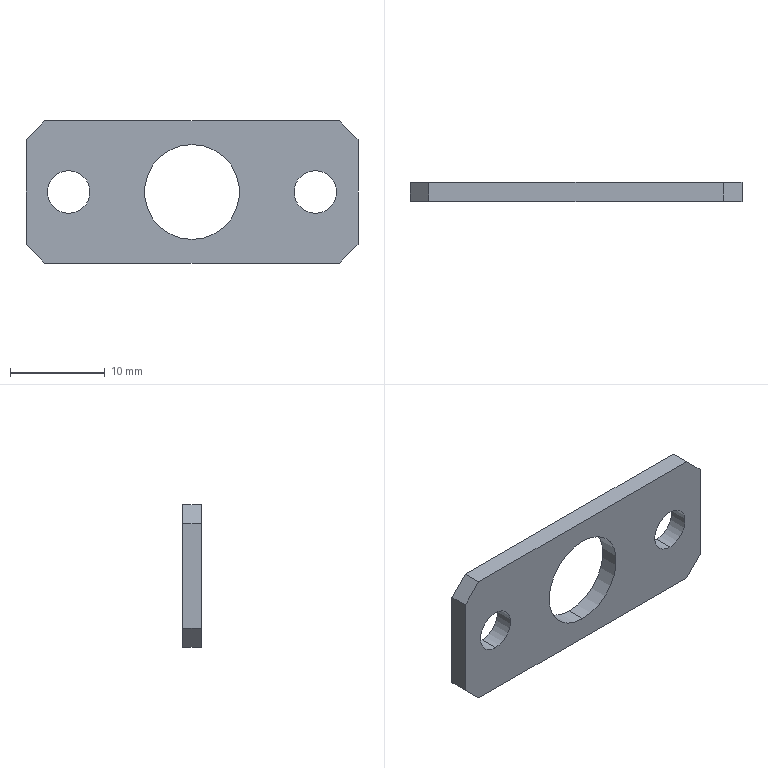Part | STEP file | 09-30 joint adapter plate (Default) | 1 solid | 16 faces | box 35 x 2 x 15 mm | volume 813.303 mm3 | plane 10 | cylinder 6 | commonest cylinder face diameters 4.5 x4 10 x2
STEP:
#1=CARTESIAN_POINT('',(13.,0.,-2.25));
#2=VERTEX_POINT('',#1);
#3=CARTESIAN_POINT('',(13.,0.,2.25));
#4=VERTEX_POINT('',#3);
#5=CARTESIAN_POINT('',(13.,0.,0.));
#6=DIRECTION('',(0.,1.,0.));
#7=DIRECTION('',(0.,0.,1.));
#8=AXIS2_PLACEMENT_3D('',#5,#6,#7);
#9=CIRCLE('',#8,2.25);
#10=EDGE_CURVE('',#2,#4,#9,.T.);
#11=ORIENTED_EDGE('',*,*,#10,.T.);
#12=CARTESIAN_POINT('',(13.,-2.,2.25));
#13=VERTEX_POINT('',#12);
#14=CARTESIAN_POINT('',(13.,8.,2.25));
#15=DIRECTION('',(0.,-1.,0.));
#16=VECTOR('',#15,1000.);
#17=LINE('',#14,#16);
#18=EDGE_CURVE('',#4,#13,#17,.T.);
#19=ORIENTED_EDGE('',*,*,#18,.T.);
#20=CARTESIAN_POINT('',(13.,-2.,-2.25));
#21=VERTEX_POINT('',#20);
#22=CARTESIAN_POINT('',(13.,-2.,0.));
#23=DIRECTION('',(0.,-1.,0.));
#24=DIRECTION('',(0.,0.,1.));
#25=AXIS2_PLACEMENT_3D('',#22,#23,#24);
#26=CIRCLE('',#25,2.25);
#27=EDGE_CURVE('',#13,#21,#26,.T.);
#28=ORIENTED_EDGE('',*,*,#27,.T.);
#29=CARTESIAN_POINT('',(13.,8.,-2.25));
#30=DIRECTION('',(0.,-1.,0.));
#31=VECTOR('',#30,1000.);
#32=LINE('',#29,#31);
#33=EDGE_CURVE('',#2,#21,#32,.T.);
#34=ORIENTED_EDGE('',*,*,#33,.F.);
#35=EDGE_LOOP('',(#11,#19,#28,#34));
#36=FACE_OUTER_BOUND('',#35,.T.);
#37=CARTESIAN_POINT('',(13.,8.,0.));
#38=DIRECTION('',(0.,-1.,0.));
#39=DIRECTION('',(0.,0.,-1.));
#40=AXIS2_PLACEMENT_3D('',#37,#38,#39);
#41=CYLINDRICAL_SURFACE('',#40,2.25);
#42=ADVANCED_FACE('',(#36),#41,.F.);
#43=CARTESIAN_POINT('',(-13.,0.,-2.25));
#44=VERTEX_POINT('',#43);
#45=CARTESIAN_POINT('',(-13.,0.,2.25));
#46=VERTEX_POINT('',#45);
#47=CARTESIAN_POINT('',(-13.,0.,0.));
#48=DIRECTION('',(0.,1.,0.));
#49=DIRECTION('',(0.,0.,1.));
#50=AXIS2_PLACEMENT_3D('',#47,#48,#49);
#51=CIRCLE('',#50,2.25);
#52=EDGE_CURVE('',#44,#46,#51,.T.);
#53=ORIENTED_EDGE('',*,*,#52,.T.);
#54=CARTESIAN_POINT('',(-13.,-2.,2.25));
#55=VERTEX_POINT('',#54);
#56=CARTESIAN_POINT('',(-13.,8.,2.25));
#57=DIRECTION('',(0.,-1.,0.));
#58=VECTOR('',#57,1000.);
#59=LINE('',#56,#58);
#60=EDGE_CURVE('',#46,#55,#59,.T.);
#61=ORIENTED_EDGE('',*,*,#60,.T.);
#62=CARTESIAN_POINT('',(-13.,-2.,-2.25));
#63=VERTEX_POINT('',#62);
#64=CARTESIAN_POINT('',(-13.,-2.,0.));
#65=DIRECTION('',(0.,-1.,0.));
#66=DIRECTION('',(0.,0.,-1.));
#67=AXIS2_PLACEMENT_3D('',#64,#65,#66);
#68=CIRCLE('',#67,2.25);
#69=EDGE_CURVE('',#55,#63,#68,.T.);
#70=ORIENTED_EDGE('',*,*,#69,.T.);
#71=CARTESIAN_POINT('',(-13.,8.,-2.25));
#72=DIRECTION('',(0.,-1.,0.));
#73=VECTOR('',#72,1000.);
#74=LINE('',#71,#73);
#75=EDGE_CURVE('',#44,#63,#74,.T.);
#76=ORIENTED_EDGE('',*,*,#75,.F.);
#77=EDGE_LOOP('',(#53,#61,#70,#76));
#78=FACE_OUTER_BOUND('',#77,.T.);
#79=CARTESIAN_POINT('',(-13.,8.,0.));
#80=DIRECTION('',(0.,-1.,0.));
#81=DIRECTION('',(0.,0.,-1.));
#82=AXIS2_PLACEMENT_3D('',#79,#80,#81);
#83=CYLINDRICAL_SURFACE('',#82,2.25);
#84=ADVANCED_FACE('',(#78),#83,.F.);
#85=CARTESIAN_POINT('',(0.,0.,-5.));
#86=VERTEX_POINT('',#85);
#87=CARTESIAN_POINT('',(0.,0.,5.));
#88=VERTEX_POINT('',#87);
#89=CARTESIAN_POINT('',(0.,0.,0.));
#90=DIRECTION('',(0.,1.,0.));
#91=DIRECTION('',(0.,0.,1.));
#92=AXIS2_PLACEMENT_3D('',#89,#90,#91);
#93=CIRCLE('',#92,5.);
#94=EDGE_CURVE('',#86,#88,#93,.T.);
#95=ORIENTED_EDGE('',*,*,#94,.T.);
#96=CARTESIAN_POINT('',(0.,-2.,5.));
#97=VERTEX_POINT('',#96);
#98=CARTESIAN_POINT('',(0.,8.,5.));
#99=DIRECTION('',(0.,-1.,0.));
#100=VECTOR('',#99,1000.);
#101=LINE('',#98,#100);
#102=EDGE_CURVE('',#88,#97,#101,.T.);
#103=ORIENTED_EDGE('',*,*,#102,.T.);
#104=CARTESIAN_POINT('',(0.,-2.,-5.));
#105=VERTEX_POINT('',#104);
#106=CARTESIAN_POINT('',(0.,-2.,0.));
#107=DIRECTION('',(0.,-1.,0.));
#108=DIRECTION('',(0.,0.,-1.));
#109=AXIS2_PLACEMENT_3D('',#106,#107,#108);
#110=CIRCLE('',#109,5.);
#111=EDGE_CURVE('',#97,#105,#110,.T.);
#112=ORIENTED_EDGE('',*,*,#111,.T.);
#113=CARTESIAN_POINT('',(0.,8.,-5.));
#114=DIRECTION('',(0.,-1.,0.));
#115=VECTOR('',#114,1000.);
#116=LINE('',#113,#115);
#117=EDGE_CURVE('',#86,#105,#116,.T.);
#118=ORIENTED_EDGE('',*,*,#117,.F.);
#119=EDGE_LOOP('',(#95,#103,#112,#118));
#120=FACE_OUTER_BOUND('',#119,.T.);
#121=CARTESIAN_POINT('',(0.,8.,0.));
#122=DIRECTION('',(0.,-1.,0.));
#123=DIRECTION('',(0.,0.,-1.));
#124=AXIS2_PLACEMENT_3D('',#121,#122,#123);
#125=CYLINDRICAL_SURFACE('',#124,5.);
#126=ADVANCED_FACE('',(#120),#125,.F.);
#127=CARTESIAN_POINT('',(17.5,-2.,5.5));
#128=VERTEX_POINT('',#127);
#129=CARTESIAN_POINT('',(17.5,-2.,-5.5));
#130=VERTEX_POINT('',#129);
#131=CARTESIAN_POINT('',(17.5,-2.,-7.5));
#132=DIRECTION('',(0.,0.,-1.));
#133=VECTOR('',#132,1000.);
#134=LINE('',#131,#133);
#135=EDGE_CURVE('',#128,#130,#134,.T.);
#136=ORIENTED_EDGE('',*,*,#135,.T.);
#137=CARTESIAN_POINT('',(17.5,0.,-5.5));
#138=VERTEX_POINT('',#137);
#139=CARTESIAN_POINT('',(17.5,-2.,-5.5));
#140=DIRECTION('',(0.,1.,0.));
#141=VECTOR('',#140,1000.);
#142=LINE('',#139,#141);
#143=EDGE_CURVE('',#130,#138,#142,.T.);
#144=ORIENTED_EDGE('',*,*,#143,.T.);
#145=CARTESIAN_POINT('',(17.5,0.,5.5));
#146=VERTEX_POINT('',#145);
#147=CARTESIAN_POINT('',(17.5,0.,-7.5));
#148=DIRECTION('',(0.,0.,-1.));
#149=VECTOR('',#148,1000.);
#150=LINE('',#147,#149);
#151=EDGE_CURVE('',#146,#138,#150,.T.);
#152=ORIENTED_EDGE('',*,*,#151,.F.);
#153=CARTESIAN_POINT('',(17.5,-2.,5.5));
#154=DIRECTION('',(0.,-1.,0.));
#155=VECTOR('',#154,1000.);
#156=LINE('',#153,#155);
#157=EDGE_CURVE('',#146,#128,#156,.T.);
#158=ORIENTED_EDGE('',*,*,#157,.T.);
#159=EDGE_LOOP('',(#136,#144,#152,#158));
#160=FACE_OUTER_BOUND('',#159,.T.);
#161=CARTESIAN_POINT('',(17.5,-2.,-7.5));
#162=DIRECTION('',(1.,0.,0.));
#163=DIRECTION('',(0.,0.,-1.));
#164=AXIS2_PLACEMENT_3D('',#161,#162,#163);
#165=PLANE('',#164);
#166=ADVANCED_FACE('',(#160),#165,.T.);
#167=CARTESIAN_POINT('',(-15.5,-2.,7.5));
#168=VERTEX_POINT('',#167);
#169=CARTESIAN_POINT('',(15.5,-2.,7.5));
#170=VERTEX_POINT('',#169);
#171=CARTESIAN_POINT('',(-17.5,-2.,7.5));
#172=DIRECTION('',(1.,0.,0.));
#173=VECTOR('',#172,1000.);
#174=LINE('',#171,#173);
#175=EDGE_CURVE('',#168,#170,#174,.T.);
#176=ORIENTED_EDGE('',*,*,#175,.T.);
#177=CARTESIAN_POINT('',(15.5,0.,7.5));
#178=VERTEX_POINT('',#177);
#179=CARTESIAN_POINT('',(15.5,-2.,7.5));
#180=DIRECTION('',(0.,1.,0.));
#181=VECTOR('',#180,1000.);
#182=LINE('',#179,#181);
#183=EDGE_CURVE('',#170,#178,#182,.T.);
#184=ORIENTED_EDGE('',*,*,#183,.T.);
#185=CARTESIAN_POINT('',(-15.5,0.,7.5));
#186=VERTEX_POINT('',#185);
#187=CARTESIAN_POINT('',(-17.5,0.,7.5));
#188=DIRECTION('',(1.,0.,0.));
#189=VECTOR('',#188,1000.);
#190=LINE('',#187,#189);
#191=EDGE_CURVE('',#186,#178,#190,.T.);
#192=ORIENTED_EDGE('',*,*,#191,.F.);
#193=CARTESIAN_POINT('',(-15.5,-2.,7.5));
#194=DIRECTION('',(0.,-1.,0.));
#195=VECTOR('',#194,1000.);
#196=LINE('',#193,#195);
#197=EDGE_CURVE('',#186,#168,#196,.T.);
#198=ORIENTED_EDGE('',*,*,#197,.T.);
#199=EDGE_LOOP('',(#176,#184,#192,#198));
#200=FACE_OUTER_BOUND('',#199,.T.);
#201=CARTESIAN_POINT('',(-17.5,-2.,7.5));
#202=DIRECTION('',(0.,0.,1.));
#203=DIRECTION('',(1.,0.,0.));
#204=AXIS2_PLACEMENT_3D('',#201,#202,#203);
#205=PLANE('',#204);
#206=ADVANCED_FACE('',(#200),#205,.T.);
#207=CARTESIAN_POINT('',(-17.5,0.,-5.5));
#208=VERTEX_POINT('',#207);
#209=CARTESIAN_POINT('',(-17.5,0.,5.5));
#210=VERTEX_POINT('',#209);
#211=CARTESIAN_POINT('',(-17.5,0.,-7.5));
#212=DIRECTION('',(0.,0.,1.));
#213=VECTOR('',#212,1000.);
#214=LINE('',#211,#213);
#215=EDGE_CURVE('',#208,#210,#214,.T.);
#216=ORIENTED_EDGE('',*,*,#215,.F.);
#217=CARTESIAN_POINT('',(-17.5,-2.,-5.5));
#218=VERTEX_POINT('',#217);
#219=CARTESIAN_POINT('',(-17.5,-2.,-5.5));
#220=DIRECTION('',(0.,-1.,0.));
#221=VECTOR('',#220,1000.);
#222=LINE('',#219,#221);
#223=EDGE_CURVE('',#208,#218,#222,.T.);
#224=ORIENTED_EDGE('',*,*,#223,.T.);
#225=CARTESIAN_POINT('',(-17.5,-2.,5.5));
#226=VERTEX_POINT('',#225);
#227=CARTESIAN_POINT('',(-17.5,-2.,-7.5));
#228=DIRECTION('',(0.,0.,1.));
#229=VECTOR('',#228,1000.);
#230=LINE('',#227,#229);
#231=EDGE_CURVE('',#218,#226,#230,.T.);
#232=ORIENTED_EDGE('',*,*,#231,.T.);
#233=CARTESIAN_POINT('',(-17.5,-2.,5.5));
#234=DIRECTION('',(0.,1.,0.));
#235=VECTOR('',#234,1000.);
#236=LINE('',#233,#235);
#237=EDGE_CURVE('',#226,#210,#236,.T.);
#238=ORIENTED_EDGE('',*,*,#237,.T.);
#239=EDGE_LOOP('',(#216,#224,#232,#238));
#240=FACE_OUTER_BOUND('',#239,.T.);
#241=CARTESIAN_POINT('',(-17.5,-2.,-7.5));
#242=DIRECTION('',(-1.,0.,0.));
#243=DIRECTION('',(0.,0.,1.));
#244=AXIS2_PLACEMENT_3D('',#241,#242,#243);
#245=PLANE('',#244);
#246=ADVANCED_FACE('',(#240),#245,.T.);
#247=CARTESIAN_POINT('',(15.5,0.,-7.5));
#248=VERTEX_POINT('',#247);
#249=CARTESIAN_POINT('',(-15.5,0.,-7.5));
#250=VERTEX_POINT('',#249);
#251=CARTESIAN_POINT('',(-17.5,0.,-7.5));
#252=DIRECTION('',(-1.,0.,0.));
#253=VECTOR('',#252,1000.);
#254=LINE('',#251,#253);
#255=EDGE_CURVE('',#248,#250,#254,.T.);
#256=ORIENTED_EDGE('',*,*,#255,.F.);
#257=CARTESIAN_POINT('',(15.5,-2.,-7.5));
#258=VERTEX_POINT('',#257);
#259=CARTESIAN_POINT('',(15.5,-2.,-7.5));
#260=DIRECTION('',(0.,-1.,0.));
#261=VECTOR('',#260,1000.);
#262=LINE('',#259,#261);
#263=EDGE_CURVE('',#248,#258,#262,.T.);
#264=ORIENTED_EDGE('',*,*,#263,.T.);
#265=CARTESIAN_POINT('',(-15.5,-2.,-7.5));
#266=VERTEX_POINT('',#265);
#267=CARTESIAN_POINT('',(-17.5,-2.,-7.5));
#268=DIRECTION('',(-1.,0.,0.));
#269=VECTOR('',#268,1000.);
#270=LINE('',#267,#269);
#271=EDGE_CURVE('',#258,#266,#270,.T.);
#272=ORIENTED_EDGE('',*,*,#271,.T.);
#273=CARTESIAN_POINT('',(-15.5,-2.,-7.5));
#274=DIRECTION('',(0.,1.,0.));
#275=VECTOR('',#274,1000.);
#276=LINE('',#273,#275);
#277=EDGE_CURVE('',#266,#250,#276,.T.);
#278=ORIENTED_EDGE('',*,*,#277,.T.);
#279=EDGE_LOOP('',(#256,#264,#272,#278));
#280=FACE_OUTER_BOUND('',#279,.T.);
#281=CARTESIAN_POINT('',(-17.5,-2.,-7.5));
#282=DIRECTION('',(0.,0.,-1.));
#283=DIRECTION('',(-1.,0.,0.));
#284=AXIS2_PLACEMENT_3D('',#281,#282,#283);
#285=PLANE('',#284);
#286=ADVANCED_FACE('',(#280),#285,.T.);
#287=CARTESIAN_POINT('',(13.,-2.,0.));
#288=DIRECTION('',(0.,-1.,0.));
#289=DIRECTION('',(0.,0.,1.));
#290=AXIS2_PLACEMENT_3D('',#287,#288,#289);
#291=CIRCLE('',#290,2.25);
#292=EDGE_CURVE('',#21,#13,#291,.T.);
#293=ORIENTED_EDGE('',*,*,#292,.F.);
#294=ORIENTED_EDGE('',*,*,#27,.F.);
#295=EDGE_LOOP('',(#293,#294));
#296=FACE_BOUND('',#295,.T.);
#297=CARTESIAN_POINT('',(-13.,-2.,0.));
#298=DIRECTION('',(0.,-1.,0.));
#299=DIRECTION('',(0.,0.,-1.));
#300=AXIS2_PLACEMENT_3D('',#297,#298,#299);
#301=CIRCLE('',#300,2.25);
#302=EDGE_CURVE('',#63,#55,#301,.T.);
#303=ORIENTED_EDGE('',*,*,#302,.F.);
#304=ORIENTED_EDGE('',*,*,#69,.F.);
#305=EDGE_LOOP('',(#303,#304));
#306=FACE_BOUND('',#305,.T.);
#307=CARTESIAN_POINT('',(0.,-2.,0.));
#308=DIRECTION('',(0.,-1.,0.));
#309=DIRECTION('',(0.,0.,-1.));
#310=AXIS2_PLACEMENT_3D('',#307,#308,#309);
#311=CIRCLE('',#310,5.);
#312=EDGE_CURVE('',#105,#97,#311,.T.);
#313=ORIENTED_EDGE('',*,*,#312,.F.);
#314=ORIENTED_EDGE('',*,*,#111,.F.);
#315=EDGE_LOOP('',(#313,#314));
#316=FACE_BOUND('',#315,.T.);
#317=ORIENTED_EDGE('',*,*,#271,.F.);
#318=CARTESIAN_POINT('',(17.5,-2.,-5.5));
#319=DIRECTION('',(0.7071,0.,0.7071));
#320=VECTOR('',#319,1000.);
#321=LINE('',#318,#320);
#322=EDGE_CURVE('',#258,#130,#321,.T.);
#323=ORIENTED_EDGE('',*,*,#322,.T.);
#324=ORIENTED_EDGE('',*,*,#135,.F.);
#325=CARTESIAN_POINT('',(15.5,-2.,7.5));
#326=DIRECTION('',(-0.7071,0.,0.7071));
#327=VECTOR('',#326,1000.);
#328=LINE('',#325,#327);
#329=EDGE_CURVE('',#128,#170,#328,.T.);
#330=ORIENTED_EDGE('',*,*,#329,.T.);
#331=ORIENTED_EDGE('',*,*,#175,.F.);
#332=CARTESIAN_POINT('',(-17.5,-2.,5.5));
#333=DIRECTION('',(-0.7071,0.,-0.7071));
#334=VECTOR('',#333,1000.);
#335=LINE('',#332,#334);
#336=EDGE_CURVE('',#168,#226,#335,.T.);
#337=ORIENTED_EDGE('',*,*,#336,.T.);
#338=ORIENTED_EDGE('',*,*,#231,.F.);
#339=CARTESIAN_POINT('',(-15.5,-2.,-7.5));
#340=DIRECTION('',(0.7071,0.,-0.7071));
#341=VECTOR('',#340,1000.);
#342=LINE('',#339,#341);
#343=EDGE_CURVE('',#218,#266,#342,.T.);
#344=ORIENTED_EDGE('',*,*,#343,.T.);
#345=EDGE_LOOP('',(#317,#323,#324,#330,#331,#337,#338,#344));
#346=FACE_OUTER_BOUND('',#345,.T.);
#347=CARTESIAN_POINT('',(17.5,-2.,7.5));
#348=DIRECTION('',(0.,1.,0.));
#349=DIRECTION('',(0.,0.,1.));
#350=AXIS2_PLACEMENT_3D('',#347,#348,#349);
#351=PLANE('',#350);
#352=ADVANCED_FACE('',(#296,#306,#316,#346),#351,.F.);
#353=ORIENTED_EDGE('',*,*,#10,.F.);
#354=CARTESIAN_POINT('',(13.,0.,0.));
#355=DIRECTION('',(0.,1.,0.));
#356=DIRECTION('',(0.,0.,1.));
#357=AXIS2_PLACEMENT_3D('',#354,#355,#356);
#358=CIRCLE('',#357,2.25);
#359=EDGE_CURVE('',#4,#2,#358,.T.);
#360=ORIENTED_EDGE('',*,*,#359,.F.);
#361=EDGE_LOOP('',(#353,#360));
#362=FACE_BOUND('',#361,.T.);
#363=ORIENTED_EDGE('',*,*,#52,.F.);
#364=CARTESIAN_POINT('',(-13.,0.,0.));
#365=DIRECTION('',(0.,1.,0.));
#366=DIRECTION('',(0.,0.,1.));
#367=AXIS2_PLACEMENT_3D('',#364,#365,#366);
#368=CIRCLE('',#367,2.25);
#369=EDGE_CURVE('',#46,#44,#368,.T.);
#370=ORIENTED_EDGE('',*,*,#369,.F.);
#371=EDGE_LOOP('',(#363,#370));
#372=FACE_BOUND('',#371,.T.);
#373=ORIENTED_EDGE('',*,*,#94,.F.);
#374=CARTESIAN_POINT('',(0.,0.,0.));
#375=DIRECTION('',(0.,1.,0.));
#376=DIRECTION('',(0.,0.,1.));
#377=AXIS2_PLACEMENT_3D('',#374,#375,#376);
#378=CIRCLE('',#377,5.);
#379=EDGE_CURVE('',#88,#86,#378,.T.);
#380=ORIENTED_EDGE('',*,*,#379,.F.);
#381=EDGE_LOOP('',(#373,#380));
#382=FACE_BOUND('',#381,.T.);
#383=ORIENTED_EDGE('',*,*,#151,.T.);
#384=CARTESIAN_POINT('',(24.,0.,1.));
#385=DIRECTION('',(-0.7071,0.,-0.7071));
#386=VECTOR('',#385,1000.);
#387=LINE('',#384,#386);
#388=EDGE_CURVE('',#138,#248,#387,.T.);
#389=ORIENTED_EDGE('',*,*,#388,.T.);
#390=ORIENTED_EDGE('',*,*,#255,.T.);
#391=CARTESIAN_POINT('',(-6.5,0.,-16.5));
#392=DIRECTION('',(-0.7071,0.,0.7071));
#393=VECTOR('',#392,1000.);
#394=LINE('',#391,#393);
#395=EDGE_CURVE('',#250,#208,#394,.T.);
#396=ORIENTED_EDGE('',*,*,#395,.T.);
#397=ORIENTED_EDGE('',*,*,#215,.T.);
#398=CARTESIAN_POINT('',(1.,0.,24.));
#399=DIRECTION('',(0.7071,0.,0.7071));
#400=VECTOR('',#399,1000.);
#401=LINE('',#398,#400);
#402=EDGE_CURVE('',#210,#186,#401,.T.);
#403=ORIENTED_EDGE('',*,*,#402,.T.);
#404=ORIENTED_EDGE('',*,*,#191,.T.);
#405=CARTESIAN_POINT('',(16.5,0.,6.5));
#406=DIRECTION('',(0.7071,0.,-0.7071));
#407=VECTOR('',#406,1000.);
#408=LINE('',#405,#407);
#409=EDGE_CURVE('',#178,#146,#408,.T.);
#410=ORIENTED_EDGE('',*,*,#409,.T.);
#411=EDGE_LOOP('',(#383,#389,#390,#396,#397,#403,#404,#410));
#412=FACE_OUTER_BOUND('',#411,.T.);
#413=CARTESIAN_POINT('',(17.5,0.,7.5));
#414=DIRECTION('',(0.,1.,0.));
#415=DIRECTION('',(0.,0.,1.));
#416=AXIS2_PLACEMENT_3D('',#413,#414,#415);
#417=PLANE('',#416);
#418=ADVANCED_FACE('',(#362,#372,#382,#412),#417,.T.);
#419=ORIENTED_EDGE('',*,*,#102,.F.);
#420=ORIENTED_EDGE('',*,*,#379,.T.);
#421=ORIENTED_EDGE('',*,*,#117,.T.);
#422=ORIENTED_EDGE('',*,*,#312,.T.);
#423=EDGE_LOOP('',(#419,#420,#421,#422));
#424=FACE_OUTER_BOUND('',#423,.T.);
#425=CARTESIAN_POINT('',(0.,8.,0.));
#426=DIRECTION('',(0.,-1.,0.));
#427=DIRECTION('',(0.,0.,-1.));
#428=AXIS2_PLACEMENT_3D('',#425,#426,#427);
#429=CYLINDRICAL_SURFACE('',#428,5.);
#430=ADVANCED_FACE('',(#424),#429,.F.);
#431=ORIENTED_EDGE('',*,*,#60,.F.);
#432=ORIENTED_EDGE('',*,*,#369,.T.);
#433=ORIENTED_EDGE('',*,*,#75,.T.);
#434=ORIENTED_EDGE('',*,*,#302,.T.);
#435=EDGE_LOOP('',(#431,#432,#433,#434));
#436=FACE_OUTER_BOUND('',#435,.T.);
#437=CARTESIAN_POINT('',(-13.,8.,0.));
#438=DIRECTION('',(0.,-1.,0.));
#439=DIRECTION('',(0.,0.,-1.));
#440=AXIS2_PLACEMENT_3D('',#437,#438,#439);
#441=CYLINDRICAL_SURFACE('',#440,2.25);
#442=ADVANCED_FACE('',(#436),#441,.F.);
#443=ORIENTED_EDGE('',*,*,#18,.F.);
#444=ORIENTED_EDGE('',*,*,#359,.T.);
#445=ORIENTED_EDGE('',*,*,#33,.T.);
#446=ORIENTED_EDGE('',*,*,#292,.T.);
#447=EDGE_LOOP('',(#443,#444,#445,#446));
#448=FACE_OUTER_BOUND('',#447,.T.);
#449=CARTESIAN_POINT('',(13.,8.,0.));
#450=DIRECTION('',(0.,-1.,0.));
#451=DIRECTION('',(0.,0.,-1.));
#452=AXIS2_PLACEMENT_3D('',#449,#450,#451);
#453=CYLINDRICAL_SURFACE('',#452,2.25);
#454=ADVANCED_FACE('',(#448),#453,.F.);
#455=ORIENTED_EDGE('',*,*,#322,.F.);
#456=ORIENTED_EDGE('',*,*,#263,.F.);
#457=ORIENTED_EDGE('',*,*,#388,.F.);
#458=ORIENTED_EDGE('',*,*,#143,.F.);
#459=EDGE_LOOP('',(#455,#456,#457,#458));
#460=FACE_OUTER_BOUND('',#459,.T.);
#461=CARTESIAN_POINT('',(17.5,-2.,-5.5));
#462=DIRECTION('',(-0.7071,0.,0.7071));
#463=DIRECTION('',(0.7071,0.,0.7071));
#464=AXIS2_PLACEMENT_3D('',#461,#462,#463);
#465=PLANE('',#464);
#466=ADVANCED_FACE('',(#460),#465,.F.);
#467=ORIENTED_EDGE('',*,*,#329,.F.);
#468=ORIENTED_EDGE('',*,*,#157,.F.);
#469=ORIENTED_EDGE('',*,*,#409,.F.);
#470=ORIENTED_EDGE('',*,*,#183,.F.);
#471=EDGE_LOOP('',(#467,#468,#469,#470));
#472=FACE_OUTER_BOUND('',#471,.T.);
#473=CARTESIAN_POINT('',(15.5,-2.,7.5));
#474=DIRECTION('',(-0.7071,0.,-0.7071));
#475=DIRECTION('',(-0.7071,0.,0.7071));
#476=AXIS2_PLACEMENT_3D('',#473,#474,#475);
#477=PLANE('',#476);
#478=ADVANCED_FACE('',(#472),#477,.F.);
#479=ORIENTED_EDGE('',*,*,#343,.F.);
#480=ORIENTED_EDGE('',*,*,#223,.F.);
#481=ORIENTED_EDGE('',*,*,#395,.F.);
#482=ORIENTED_EDGE('',*,*,#277,.F.);
#483=EDGE_LOOP('',(#479,#480,#481,#482));
#484=FACE_OUTER_BOUND('',#483,.T.);
#485=CARTESIAN_POINT('',(-15.5,-2.,-7.5));
#486=DIRECTION('',(0.7071,0.,0.7071));
#487=DIRECTION('',(0.7071,0.,-0.7071));
#488=AXIS2_PLACEMENT_3D('',#485,#486,#487);
#489=PLANE('',#488);
#490=ADVANCED_FACE('',(#484),#489,.F.);
#491=ORIENTED_EDGE('',*,*,#336,.F.);
#492=ORIENTED_EDGE('',*,*,#197,.F.);
#493=ORIENTED_EDGE('',*,*,#402,.F.);
#494=ORIENTED_EDGE('',*,*,#237,.F.);
#495=EDGE_LOOP('',(#491,#492,#493,#494));
#496=FACE_OUTER_BOUND('',#495,.T.);
#497=CARTESIAN_POINT('',(-17.5,-2.,5.5));
#498=DIRECTION('',(0.7071,0.,-0.7071));
#499=DIRECTION('',(-0.7071,0.,-0.7071));
#500=AXIS2_PLACEMENT_3D('',#497,#498,#499);
#501=PLANE('',#500);
#502=ADVANCED_FACE('',(#496),#501,.F.);
#503=CLOSED_SHELL('',(#42,#84,#126,#166,#206,#246,#286,#352,#418,#430,#442,#454,#466,#478,#490,#502));
#504=MANIFOLD_SOLID_BREP('',#503);
#505=CARTESIAN_POINT('',(0.,0.,0.));
#506=DIRECTION('',(0.,0.,1.));
#507=DIRECTION('',(1.,0.,0.));
#508=AXIS2_PLACEMENT_3D('',#505,#506,#507);
#509=(LENGTH_UNIT()NAMED_UNIT(*)SI_UNIT(.MILLI.,.METRE.));
#510=UNCERTAINTY_MEASURE_WITH_UNIT(LENGTH_MEASURE(0.00001),#509,'','');
#511=(NAMED_UNIT(*)PLANE_ANGLE_UNIT()SI_UNIT($,.RADIAN.));
#512=(NAMED_UNIT(*)SI_UNIT($,.STERADIAN.)SOLID_ANGLE_UNIT());
#513=(GEOMETRIC_REPRESENTATION_CONTEXT(3)GLOBAL_UNCERTAINTY_ASSIGNED_CONTEXT((#510))GLOBAL_UNIT_ASSIGNED_CONTEXT((#509,#511,#512))REPRESENTATION_CONTEXT('',''));
#514=ADVANCED_BREP_SHAPE_REPRESENTATION('',(#504,#508),#513);